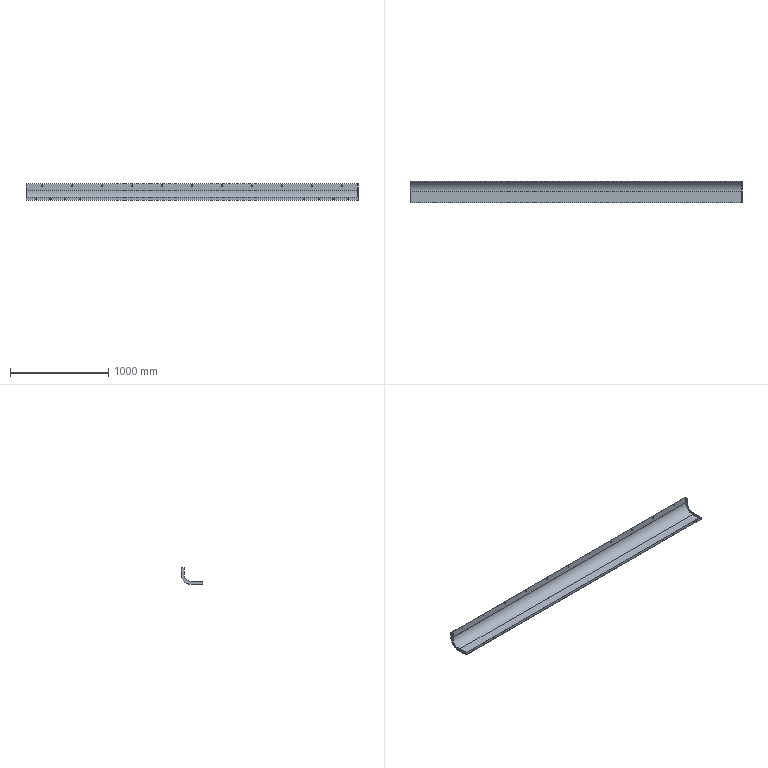Part | NX | features BREP 3 | 3 solids | 131 faces | box 3380 x 220 x 170 mm | volume 1917418 mm3 | plane 72 | cylinder 59 | commonest cylinder face diameters 7 x34 6 x16 4 x3 197 x3 140 x2 200 x1